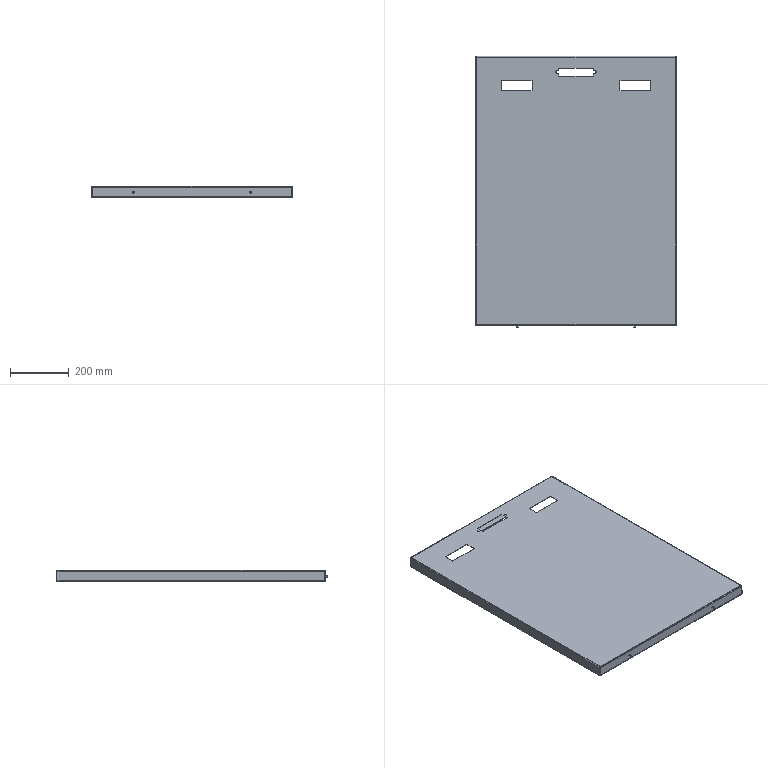Part | SolidWorks | features ICE 6, SMWeldBead 4, EdgeFlange 2, FlatPattern 1, HoleWzd 1, SMBaseFlange 1, SheetMetal 1 | 1 solid | 145 faces | box 685 x 925 x 38 mm | volume 1199110 mm3 | plane 76 | spline 40 | cylinder 29 | commonest cylinder face diameters 4 x8 7 x8 6 x6 2 x4 9 x3